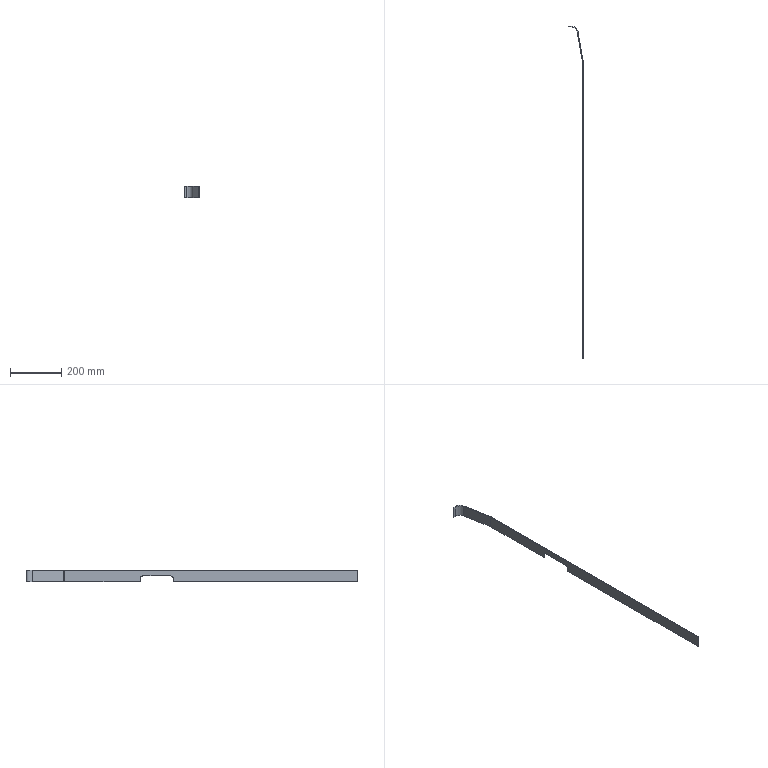Part | SolidWorks | features FlatPattern 1, ICE 1, SMBaseFlange 1, SheetMetal 1 | 1 solid | 28 faces | box 60.1 x 1293 x 45 mm | volume 180831 mm3 | plane 22 | cylinder 6 | commonest cylinder face diameters 20 x2 50 x2 56.4 x2
STEP:
#1=CARTESIAN_POINT('',(63.4,-447.3,-22.5));
#2=VERTEX_POINT('',#1);
#3=CARTESIAN_POINT('',(60.2,-447.3,-22.5));
#4=VERTEX_POINT('',#3);
#5=CARTESIAN_POINT('',(63.4,-447.3,-22.5));
#6=DIRECTION('',(-1.,0.,0.));
#7=VECTOR('',#6,1000.);
#8=LINE('',#5,#7);
#9=EDGE_CURVE('',#2,#4,#8,.T.);
#10=ORIENTED_EDGE('',*,*,#9,.T.);
#11=CARTESIAN_POINT('',(60.2,-153.273,-22.5));
#12=VERTEX_POINT('',#11);
#13=CARTESIAN_POINT('',(60.2,-153.273,-22.5));
#14=DIRECTION('',(0.,1.,0.));
#15=VECTOR('',#14,1000.);
#16=LINE('',#13,#15);
#17=EDGE_CURVE('',#4,#12,#16,.T.);
#18=ORIENTED_EDGE('',*,*,#17,.T.);
#19=CARTESIAN_POINT('',(63.4,-153.273,-22.5));
#20=VERTEX_POINT('',#19);
#21=CARTESIAN_POINT('',(60.2,-153.273,-22.5));
#22=DIRECTION('',(1.,0.,0.));
#23=VECTOR('',#22,1000.);
#24=LINE('',#21,#23);
#25=EDGE_CURVE('',#12,#20,#24,.T.);
#26=ORIENTED_EDGE('',*,*,#25,.T.);
#27=CARTESIAN_POINT('',(63.4,-153.273,-22.5));
#28=DIRECTION('',(0.,1.,0.));
#29=VECTOR('',#28,1000.);
#30=LINE('',#27,#29);
#31=EDGE_CURVE('',#2,#20,#30,.T.);
#32=ORIENTED_EDGE('',*,*,#31,.F.);
#33=EDGE_LOOP('',(#10,#18,#26,#32));
#34=FACE_OUTER_BOUND('',#33,.T.);
#35=CARTESIAN_POINT('',(62.97,-148.368,-22.5));
#36=DIRECTION('',(0.,0.,-1.));
#37=DIRECTION('',(-1.,0.,0.));
#38=AXIS2_PLACEMENT_3D('',#35,#36,#37);
#39=PLANE('',#38);
#40=ADVANCED_FACE('',(#34),#39,.T.);
#41=CARTESIAN_POINT('',(59.819,-148.925,22.5));
#42=VERTEX_POINT('',#41);
#43=CARTESIAN_POINT('',(62.97,-148.368,22.5));
#44=VERTEX_POINT('',#43);
#45=CARTESIAN_POINT('',(59.819,-148.925,22.5));
#46=DIRECTION('',(0.9848,0.1739,0.));
#47=VECTOR('',#46,1000.);
#48=LINE('',#45,#47);
#49=EDGE_CURVE('',#42,#44,#48,.T.);
#50=ORIENTED_EDGE('',*,*,#49,.F.);
#51=CARTESIAN_POINT('',(60.2,-153.273,22.5));
#52=VERTEX_POINT('',#51);
#53=CARTESIAN_POINT('',(35.2,-153.273,22.5));
#54=DIRECTION('',(0.,0.,1.));
#55=DIRECTION('',(-1.,0.,0.));
#56=AXIS2_PLACEMENT_3D('',#53,#54,#55);
#57=CIRCLE('',#56,25.);
#58=EDGE_CURVE('',#52,#42,#57,.T.);
#59=ORIENTED_EDGE('',*,*,#58,.F.);
#60=CARTESIAN_POINT('',(63.4,-153.273,22.5));
#61=VERTEX_POINT('',#60);
#62=CARTESIAN_POINT('',(63.4,-153.273,22.5));
#63=DIRECTION('',(-1.,0.,0.));
#64=VECTOR('',#63,1000.);
#65=LINE('',#62,#64);
#66=EDGE_CURVE('',#61,#52,#65,.T.);
#67=ORIENTED_EDGE('',*,*,#66,.F.);
#68=CARTESIAN_POINT('',(35.2,-153.273,22.5));
#69=DIRECTION('',(0.,0.,1.));
#70=DIRECTION('',(1.,0.,0.));
#71=AXIS2_PLACEMENT_3D('',#68,#69,#70);
#72=CIRCLE('',#71,28.2);
#73=EDGE_CURVE('',#61,#44,#72,.T.);
#74=ORIENTED_EDGE('',*,*,#73,.T.);
#75=EDGE_LOOP('',(#50,#59,#67,#74));
#76=FACE_OUTER_BOUND('',#75,.T.);
#77=CARTESIAN_POINT('',(59.819,-148.925,22.5));
#78=DIRECTION('',(0.,0.,1.));
#79=DIRECTION('',(1.,0.,0.));
#80=AXIS2_PLACEMENT_3D('',#77,#78,#79);
#81=PLANE('',#80);
#82=ADVANCED_FACE('',(#76),#81,.T.);
#83=CARTESIAN_POINT('',(38.134,-26.152,22.5));
#84=VERTEX_POINT('',#83);
#85=CARTESIAN_POINT('',(38.134,-26.152,22.5));
#86=DIRECTION('',(-0.1739,0.9848,0.));
#87=VECTOR('',#86,1000.);
#88=LINE('',#85,#87);
#89=EDGE_CURVE('',#42,#84,#88,.T.);
#90=ORIENTED_EDGE('',*,*,#89,.F.);
#91=ORIENTED_EDGE('',*,*,#49,.T.);
#92=CARTESIAN_POINT('',(41.285,-25.595,22.5));
#93=VERTEX_POINT('',#92);
#94=CARTESIAN_POINT('',(41.285,-25.595,22.5));
#95=DIRECTION('',(-0.1739,0.9848,0.));
#96=VECTOR('',#95,1000.);
#97=LINE('',#94,#96);
#98=EDGE_CURVE('',#44,#93,#97,.T.);
#99=ORIENTED_EDGE('',*,*,#98,.T.);
#100=CARTESIAN_POINT('',(41.285,-25.595,22.5));
#101=DIRECTION('',(-0.9848,-0.1739,0.));
#102=VECTOR('',#101,1000.);
#103=LINE('',#100,#102);
#104=EDGE_CURVE('',#93,#84,#103,.T.);
#105=ORIENTED_EDGE('',*,*,#104,.T.);
#106=EDGE_LOOP('',(#90,#91,#99,#105));
#107=FACE_OUTER_BOUND('',#106,.T.);
#108=CARTESIAN_POINT('',(63.4,-153.273,22.5));
#109=DIRECTION('',(0.,0.,1.));
#110=DIRECTION('',(1.,0.,0.));
#111=AXIS2_PLACEMENT_3D('',#108,#109,#110);
#112=PLANE('',#111);
#113=ADVANCED_FACE('',(#107),#112,.T.);
#114=ORIENTED_EDGE('',*,*,#25,.F.);
#115=CARTESIAN_POINT('',(59.819,-148.925,-22.5));
#116=VERTEX_POINT('',#115);
#117=CARTESIAN_POINT('',(35.2,-153.273,-22.5));
#118=DIRECTION('',(0.,0.,1.));
#119=DIRECTION('',(-1.,0.,0.));
#120=AXIS2_PLACEMENT_3D('',#117,#118,#119);
#121=CIRCLE('',#120,25.);
#122=EDGE_CURVE('',#12,#116,#121,.T.);
#123=ORIENTED_EDGE('',*,*,#122,.T.);
#124=CARTESIAN_POINT('',(62.97,-148.368,-22.5));
#125=VERTEX_POINT('',#124);
#126=CARTESIAN_POINT('',(62.97,-148.368,-22.5));
#127=DIRECTION('',(-0.9848,-0.1739,0.));
#128=VECTOR('',#127,1000.);
#129=LINE('',#126,#128);
#130=EDGE_CURVE('',#125,#116,#129,.T.);
#131=ORIENTED_EDGE('',*,*,#130,.F.);
#132=CARTESIAN_POINT('',(35.2,-153.273,-22.5));
#133=DIRECTION('',(0.,0.,1.));
#134=DIRECTION('',(1.,0.,0.));
#135=AXIS2_PLACEMENT_3D('',#132,#133,#134);
#136=CIRCLE('',#135,28.2);
#137=EDGE_CURVE('',#20,#125,#136,.T.);
#138=ORIENTED_EDGE('',*,*,#137,.F.);
#139=EDGE_LOOP('',(#114,#123,#131,#138));
#140=FACE_OUTER_BOUND('',#139,.T.);
#141=CARTESIAN_POINT('',(60.2,-153.273,-22.5));
#142=DIRECTION('',(0.,0.,-1.));
#143=DIRECTION('',(-1.,0.,0.));
#144=AXIS2_PLACEMENT_3D('',#141,#142,#143);
#145=PLANE('',#144);
#146=ADVANCED_FACE('',(#140),#145,.T.);
#147=CARTESIAN_POINT('',(63.4,-575.3,-22.5));
#148=VERTEX_POINT('',#147);
#149=CARTESIAN_POINT('',(60.2,-575.3,-22.5));
#150=VERTEX_POINT('',#149);
#151=CARTESIAN_POINT('',(63.4,-575.3,-22.5));
#152=DIRECTION('',(-1.,0.,0.));
#153=VECTOR('',#152,1000.);
#154=LINE('',#151,#153);
#155=EDGE_CURVE('',#148,#150,#154,.T.);
#156=ORIENTED_EDGE('',*,*,#155,.F.);
#157=CARTESIAN_POINT('',(63.4,-1295.7,-22.5));
#158=VERTEX_POINT('',#157);
#159=CARTESIAN_POINT('',(63.4,-153.273,-22.5));
#160=DIRECTION('',(0.,1.,0.));
#161=VECTOR('',#160,1000.);
#162=LINE('',#159,#161);
#163=EDGE_CURVE('',#158,#148,#162,.T.);
#164=ORIENTED_EDGE('',*,*,#163,.F.);
#165=CARTESIAN_POINT('',(60.2,-1295.7,-22.5));
#166=VERTEX_POINT('',#165);
#167=CARTESIAN_POINT('',(63.4,-1295.7,-22.5));
#168=DIRECTION('',(-1.,0.,0.));
#169=VECTOR('',#168,1000.);
#170=LINE('',#167,#169);
#171=EDGE_CURVE('',#158,#166,#170,.T.);
#172=ORIENTED_EDGE('',*,*,#171,.T.);
#173=CARTESIAN_POINT('',(60.2,-153.273,-22.5));
#174=DIRECTION('',(0.,1.,0.));
#175=VECTOR('',#174,1000.);
#176=LINE('',#173,#175);
#177=EDGE_CURVE('',#166,#150,#176,.T.);
#178=ORIENTED_EDGE('',*,*,#177,.T.);
#179=EDGE_LOOP('',(#156,#164,#172,#178));
#180=FACE_OUTER_BOUND('',#179,.T.);
#181=CARTESIAN_POINT('',(62.97,-148.368,-22.5));
#182=DIRECTION('',(0.,0.,-1.));
#183=DIRECTION('',(-1.,0.,0.));
#184=AXIS2_PLACEMENT_3D('',#181,#182,#183);
#185=PLANE('',#184);
#186=ADVANCED_FACE('',(#180),#185,.T.);
#187=CARTESIAN_POINT('',(13.515,-5.5,22.5));
#188=VERTEX_POINT('',#187);
#189=CARTESIAN_POINT('',(13.515,-2.3,22.5));
#190=VERTEX_POINT('',#189);
#191=CARTESIAN_POINT('',(13.515,-5.5,22.5));
#192=DIRECTION('',(0.,1.,0.));
#193=VECTOR('',#192,1000.);
#194=LINE('',#191,#193);
#195=EDGE_CURVE('',#188,#190,#194,.T.);
#196=ORIENTED_EDGE('',*,*,#195,.F.);
#197=CARTESIAN_POINT('',(13.515,-30.5,22.5));
#198=DIRECTION('',(0.,0.,1.));
#199=DIRECTION('',(-1.,0.,0.));
#200=AXIS2_PLACEMENT_3D('',#197,#198,#199);
#201=CIRCLE('',#200,25.);
#202=EDGE_CURVE('',#84,#188,#201,.T.);
#203=ORIENTED_EDGE('',*,*,#202,.F.);
#204=ORIENTED_EDGE('',*,*,#104,.F.);
#205=CARTESIAN_POINT('',(13.515,-30.5,22.5));
#206=DIRECTION('',(0.,0.,1.));
#207=DIRECTION('',(1.,0.,0.));
#208=AXIS2_PLACEMENT_3D('',#205,#206,#207);
#209=CIRCLE('',#208,28.2);
#210=EDGE_CURVE('',#93,#190,#209,.T.);
#211=ORIENTED_EDGE('',*,*,#210,.T.);
#212=EDGE_LOOP('',(#196,#203,#204,#211));
#213=FACE_OUTER_BOUND('',#212,.T.);
#214=CARTESIAN_POINT('',(13.515,-5.5,22.5));
#215=DIRECTION('',(0.,0.,1.));
#216=DIRECTION('',(1.,0.,0.));
#217=AXIS2_PLACEMENT_3D('',#214,#215,#216);
#218=PLANE('',#217);
#219=ADVANCED_FACE('',(#213),#218,.T.);
#220=CARTESIAN_POINT('',(3.3,-5.5,22.5));
#221=VERTEX_POINT('',#220);
#222=CARTESIAN_POINT('',(13.515,-5.5,22.5));
#223=DIRECTION('',(-1.,0.,0.));
#224=VECTOR('',#223,1000.);
#225=LINE('',#222,#224);
#226=EDGE_CURVE('',#188,#221,#225,.T.);
#227=ORIENTED_EDGE('',*,*,#226,.F.);
#228=ORIENTED_EDGE('',*,*,#195,.T.);
#229=CARTESIAN_POINT('',(3.3,-2.3,22.5));
#230=VERTEX_POINT('',#229);
#231=CARTESIAN_POINT('',(13.515,-2.3,22.5));
#232=DIRECTION('',(-1.,0.,0.));
#233=VECTOR('',#232,1000.);
#234=LINE('',#231,#233);
#235=EDGE_CURVE('',#190,#230,#234,.T.);
#236=ORIENTED_EDGE('',*,*,#235,.T.);
#237=CARTESIAN_POINT('',(3.3,-5.5,22.5));
#238=DIRECTION('',(0.,1.,0.));
#239=VECTOR('',#238,1000.);
#240=LINE('',#237,#239);
#241=EDGE_CURVE('',#221,#230,#240,.T.);
#242=ORIENTED_EDGE('',*,*,#241,.F.);
#243=EDGE_LOOP('',(#227,#228,#236,#242));
#244=FACE_OUTER_BOUND('',#243,.T.);
#245=CARTESIAN_POINT('',(41.285,-25.595,22.5));
#246=DIRECTION('',(0.,0.,1.));
#247=DIRECTION('',(1.,0.,0.));
#248=AXIS2_PLACEMENT_3D('',#245,#246,#247);
#249=PLANE('',#248);
#250=ADVANCED_FACE('',(#244),#249,.T.);
#251=CARTESIAN_POINT('',(38.134,-26.152,-22.5));
#252=VERTEX_POINT('',#251);
#253=CARTESIAN_POINT('',(41.285,-25.595,-22.5));
#254=VERTEX_POINT('',#253);
#255=CARTESIAN_POINT('',(38.134,-26.152,-22.5));
#256=DIRECTION('',(0.9848,0.1739,0.));
#257=VECTOR('',#256,1000.);
#258=LINE('',#255,#257);
#259=EDGE_CURVE('',#252,#254,#258,.T.);
#260=ORIENTED_EDGE('',*,*,#259,.F.);
#261=CARTESIAN_POINT('',(13.515,-5.5,-22.5));
#262=VERTEX_POINT('',#261);
#263=CARTESIAN_POINT('',(13.515,-30.5,-22.5));
#264=DIRECTION('',(0.,0.,1.));
#265=DIRECTION('',(-1.,0.,0.));
#266=AXIS2_PLACEMENT_3D('',#263,#264,#265);
#267=CIRCLE('',#266,25.);
#268=EDGE_CURVE('',#252,#262,#267,.T.);
#269=ORIENTED_EDGE('',*,*,#268,.T.);
#270=CARTESIAN_POINT('',(13.515,-2.3,-22.5));
#271=VERTEX_POINT('',#270);
#272=CARTESIAN_POINT('',(13.515,-2.3,-22.5));
#273=DIRECTION('',(0.,-1.,0.));
#274=VECTOR('',#273,1000.);
#275=LINE('',#272,#274);
#276=EDGE_CURVE('',#271,#262,#275,.T.);
#277=ORIENTED_EDGE('',*,*,#276,.F.);
#278=CARTESIAN_POINT('',(13.515,-30.5,-22.5));
#279=DIRECTION('',(0.,0.,1.));
#280=DIRECTION('',(1.,0.,0.));
#281=AXIS2_PLACEMENT_3D('',#278,#279,#280);
#282=CIRCLE('',#281,28.2);
#283=EDGE_CURVE('',#254,#271,#282,.T.);
#284=ORIENTED_EDGE('',*,*,#283,.F.);
#285=EDGE_LOOP('',(#260,#269,#277,#284));
#286=FACE_OUTER_BOUND('',#285,.T.);
#287=CARTESIAN_POINT('',(38.134,-26.152,-22.5));
#288=DIRECTION('',(0.,0.,-1.));
#289=DIRECTION('',(-1.,0.,0.));
#290=AXIS2_PLACEMENT_3D('',#287,#288,#289);
#291=PLANE('',#290);
#292=ADVANCED_FACE('',(#286),#291,.T.);
#293=CARTESIAN_POINT('',(38.134,-26.152,-22.5));
#294=DIRECTION('',(-0.1739,0.9848,0.));
#295=VECTOR('',#294,1000.);
#296=LINE('',#293,#295);
#297=EDGE_CURVE('',#116,#252,#296,.T.);
#298=ORIENTED_EDGE('',*,*,#297,.T.);
#299=ORIENTED_EDGE('',*,*,#259,.T.);
#300=CARTESIAN_POINT('',(41.285,-25.595,-22.5));
#301=DIRECTION('',(-0.1739,0.9848,0.));
#302=VECTOR('',#301,1000.);
#303=LINE('',#300,#302);
#304=EDGE_CURVE('',#125,#254,#303,.T.);
#305=ORIENTED_EDGE('',*,*,#304,.F.);
#306=ORIENTED_EDGE('',*,*,#130,.T.);
#307=EDGE_LOOP('',(#298,#299,#305,#306));
#308=FACE_OUTER_BOUND('',#307,.T.);
#309=CARTESIAN_POINT('',(13.515,-2.3,-22.5));
#310=DIRECTION('',(0.,0.,-1.));
#311=DIRECTION('',(-1.,0.,0.));
#312=AXIS2_PLACEMENT_3D('',#309,#310,#311);
#313=PLANE('',#312);
#314=ADVANCED_FACE('',(#308),#313,.T.);
#315=CARTESIAN_POINT('',(3.3,-2.3,-22.5));
#316=VERTEX_POINT('',#315);
#317=CARTESIAN_POINT('',(13.515,-2.3,-22.5));
#318=DIRECTION('',(-1.,0.,0.));
#319=VECTOR('',#318,1000.);
#320=LINE('',#317,#319);
#321=EDGE_CURVE('',#271,#316,#320,.T.);
#322=ORIENTED_EDGE('',*,*,#321,.T.);
#323=CARTESIAN_POINT('',(3.3,-2.3,22.5));
#324=DIRECTION('',(0.,0.,-1.));
#325=VECTOR('',#324,1000.);
#326=LINE('',#323,#325);
#327=EDGE_CURVE('',#230,#316,#326,.T.);
#328=ORIENTED_EDGE('',*,*,#327,.F.);
#329=ORIENTED_EDGE('',*,*,#235,.F.);
#330=CARTESIAN_POINT('',(13.515,-2.3,22.5));
#331=DIRECTION('',(0.,0.,-1.));
#332=VECTOR('',#331,1000.);
#333=LINE('',#330,#332);
#334=EDGE_CURVE('',#190,#271,#333,.T.);
#335=ORIENTED_EDGE('',*,*,#334,.T.);
#336=EDGE_LOOP('',(#322,#328,#329,#335));
#337=FACE_OUTER_BOUND('',#336,.T.);
#338=CARTESIAN_POINT('',(13.515,-2.3,22.5));
#339=DIRECTION('',(0.,-1.,0.));
#340=DIRECTION('',(1.,0.,0.));
#341=AXIS2_PLACEMENT_3D('',#338,#339,#340);
#342=PLANE('',#341);
#343=ADVANCED_FACE('',(#337),#342,.F.);
#344=CARTESIAN_POINT('',(3.3,-5.5,-22.5));
#345=VERTEX_POINT('',#344);
#346=CARTESIAN_POINT('',(3.3,-5.5,-22.5));
#347=DIRECTION('',(0.,1.,0.));
#348=VECTOR('',#347,1000.);
#349=LINE('',#346,#348);
#350=EDGE_CURVE('',#345,#316,#349,.T.);
#351=ORIENTED_EDGE('',*,*,#350,.F.);
#352=CARTESIAN_POINT('',(3.3,-5.5,22.5));
#353=DIRECTION('',(0.,0.,-1.));
#354=VECTOR('',#353,1000.);
#355=LINE('',#352,#354);
#356=EDGE_CURVE('',#221,#345,#355,.T.);
#357=ORIENTED_EDGE('',*,*,#356,.F.);
#358=ORIENTED_EDGE('',*,*,#241,.T.);
#359=ORIENTED_EDGE('',*,*,#327,.T.);
#360=EDGE_LOOP('',(#351,#357,#358,#359));
#361=FACE_OUTER_BOUND('',#360,.T.);
#362=CARTESIAN_POINT('',(3.3,-5.5,22.5));
#363=DIRECTION('',(-1.,0.,0.));
#364=DIRECTION('',(0.,0.,1.));
#365=AXIS2_PLACEMENT_3D('',#362,#363,#364);
#366=PLANE('',#365);
#367=ADVANCED_FACE('',(#361),#366,.T.);
#368=CARTESIAN_POINT('',(13.515,-5.5,-22.5));
#369=DIRECTION('',(-1.,0.,0.));
#370=VECTOR('',#369,1000.);
#371=LINE('',#368,#370);
#372=EDGE_CURVE('',#262,#345,#371,.T.);
#373=ORIENTED_EDGE('',*,*,#372,.F.);
#374=CARTESIAN_POINT('',(13.515,-5.5,22.5));
#375=DIRECTION('',(0.,0.,-1.));
#376=VECTOR('',#375,1000.);
#377=LINE('',#374,#376);
#378=EDGE_CURVE('',#188,#262,#377,.T.);
#379=ORIENTED_EDGE('',*,*,#378,.F.);
#380=ORIENTED_EDGE('',*,*,#226,.T.);
#381=ORIENTED_EDGE('',*,*,#356,.T.);
#382=EDGE_LOOP('',(#373,#379,#380,#381));
#383=FACE_OUTER_BOUND('',#382,.T.);
#384=CARTESIAN_POINT('',(13.515,-5.5,22.5));
#385=DIRECTION('',(0.,-1.,0.));
#386=DIRECTION('',(1.,0.,0.));
#387=AXIS2_PLACEMENT_3D('',#384,#385,#386);
#388=PLANE('',#387);
#389=ADVANCED_FACE('',(#383),#388,.T.);
#390=ORIENTED_EDGE('',*,*,#268,.F.);
#391=CARTESIAN_POINT('',(38.134,-26.152,22.5));
#392=DIRECTION('',(0.,0.,-1.));
#393=VECTOR('',#392,1000.);
#394=LINE('',#391,#393);
#395=EDGE_CURVE('',#84,#252,#394,.T.);
#396=ORIENTED_EDGE('',*,*,#395,.F.);
#397=ORIENTED_EDGE('',*,*,#202,.T.);
#398=ORIENTED_EDGE('',*,*,#378,.T.);
#399=EDGE_LOOP('',(#390,#396,#397,#398));
#400=FACE_OUTER_BOUND('',#399,.T.);
#401=CARTESIAN_POINT('',(13.515,-30.5,22.5));
#402=DIRECTION('',(0.,0.,-1.));
#403=DIRECTION('',(-1.,0.,0.));
#404=AXIS2_PLACEMENT_3D('',#401,#402,#403);
#405=CYLINDRICAL_SURFACE('',#404,25.);
#406=ADVANCED_FACE('',(#400),#405,.F.);
#407=ORIENTED_EDGE('',*,*,#297,.F.);
#408=CARTESIAN_POINT('',(59.819,-148.925,22.5));
#409=DIRECTION('',(0.,0.,-1.));
#410=VECTOR('',#409,1000.);
#411=LINE('',#408,#410);
#412=EDGE_CURVE('',#42,#116,#411,.T.);
#413=ORIENTED_EDGE('',*,*,#412,.F.);
#414=ORIENTED_EDGE('',*,*,#89,.T.);
#415=ORIENTED_EDGE('',*,*,#395,.T.);
#416=EDGE_LOOP('',(#407,#413,#414,#415));
#417=FACE_OUTER_BOUND('',#416,.T.);
#418=CARTESIAN_POINT('',(38.134,-26.152,22.5));
#419=DIRECTION('',(-0.9848,-0.1739,0.));
#420=DIRECTION('',(0.1739,-0.9848,0.));
#421=AXIS2_PLACEMENT_3D('',#418,#419,#420);
#422=PLANE('',#421);
#423=ADVANCED_FACE('',(#417),#422,.T.);
#424=ORIENTED_EDGE('',*,*,#122,.F.);
#425=CARTESIAN_POINT('',(60.2,-153.273,22.5));
#426=DIRECTION('',(0.,0.,-1.));
#427=VECTOR('',#426,1000.);
#428=LINE('',#425,#427);
#429=EDGE_CURVE('',#52,#12,#428,.T.);
#430=ORIENTED_EDGE('',*,*,#429,.F.);
#431=ORIENTED_EDGE('',*,*,#58,.T.);
#432=ORIENTED_EDGE('',*,*,#412,.T.);
#433=EDGE_LOOP('',(#424,#430,#431,#432));
#434=FACE_OUTER_BOUND('',#433,.T.);
#435=CARTESIAN_POINT('',(35.2,-153.273,22.5));
#436=DIRECTION('',(0.,0.,-1.));
#437=DIRECTION('',(-1.,0.,0.));
#438=AXIS2_PLACEMENT_3D('',#435,#436,#437);
#439=CYLINDRICAL_SURFACE('',#438,25.);
#440=ADVANCED_FACE('',(#434),#439,.F.);
#441=CARTESIAN_POINT('',(60.2,-447.3,-9.9));
#442=VERTEX_POINT('',#441);
#443=CARTESIAN_POINT('',(60.2,-447.3,-9.9));
#444=DIRECTION('',(0.,0.,-1.));
#445=VECTOR('',#444,1000.);
#446=LINE('',#443,#445);
#447=EDGE_CURVE('',#442,#4,#446,.T.);
#448=ORIENTED_EDGE('',*,*,#447,.F.);
#449=CARTESIAN_POINT('',(60.2,-457.3,0.1));
#450=VERTEX_POINT('',#449);
#451=CARTESIAN_POINT('',(60.2,-457.3,-9.9));
#452=DIRECTION('',(-1.,0.,0.));
#453=DIRECTION('',(0.,-1.,0.));
#454=AXIS2_PLACEMENT_3D('',#451,#452,#453);
#455=CIRCLE('',#454,10.);
#456=EDGE_CURVE('',#450,#442,#455,.T.);
#457=ORIENTED_EDGE('',*,*,#456,.F.);
#458=CARTESIAN_POINT('',(60.2,-565.3,0.1));
#459=VERTEX_POINT('',#458);
#460=CARTESIAN_POINT('',(60.2,-457.3,0.1));
#461=DIRECTION('',(0.,1.,0.));
#462=VECTOR('',#461,1000.);
#463=LINE('',#460,#462);
#464=EDGE_CURVE('',#459,#450,#463,.T.);
#465=ORIENTED_EDGE('',*,*,#464,.F.);
#466=CARTESIAN_POINT('',(60.2,-575.3,-9.9));
#467=VERTEX_POINT('',#466);
#468=CARTESIAN_POINT('',(60.2,-565.3,-9.9));
#469=DIRECTION('',(-1.,0.,0.));
#470=DIRECTION('',(0.,1.,0.));
#471=AXIS2_PLACEMENT_3D('',#468,#469,#470);
#472=CIRCLE('',#471,10.);
#473=EDGE_CURVE('',#467,#459,#472,.T.);
#474=ORIENTED_EDGE('',*,*,#473,.F.);
#475=CARTESIAN_POINT('',(60.2,-575.3,-22.5));
#476=DIRECTION('',(0.,0.,1.));
#477=VECTOR('',#476,1000.);
#478=LINE('',#475,#477);
#479=EDGE_CURVE('',#150,#467,#478,.T.);
#480=ORIENTED_EDGE('',*,*,#479,.F.);
#481=ORIENTED_EDGE('',*,*,#177,.F.);
#482=CARTESIAN_POINT('',(60.2,-1295.7,22.5));
#483=VERTEX_POINT('',#482);
#484=CARTESIAN_POINT('',(60.2,-1295.7,22.5));
#485=DIRECTION('',(0.,0.,-1.));
#486=VECTOR('',#485,1000.);
#487=LINE('',#484,#486);
#488=EDGE_CURVE('',#483,#166,#487,.T.);
#489=ORIENTED_EDGE('',*,*,#488,.F.);
#490=CARTESIAN_POINT('',(60.2,-153.273,22.5));
#491=DIRECTION('',(0.,1.,0.));
#492=VECTOR('',#491,1000.);
#493=LINE('',#490,#492);
#494=EDGE_CURVE('',#483,#52,#493,.T.);
#495=ORIENTED_EDGE('',*,*,#494,.T.);
#496=ORIENTED_EDGE('',*,*,#429,.T.);
#497=ORIENTED_EDGE('',*,*,#17,.F.);
#498=EDGE_LOOP('',(#448,#457,#465,#474,#480,#481,#489,#495,#496,#497));
#499=FACE_OUTER_BOUND('',#498,.T.);
#500=CARTESIAN_POINT('',(60.2,-153.273,22.5));
#501=DIRECTION('',(-1.,0.,0.));
#502=DIRECTION('',(0.,-1.,0.));
#503=AXIS2_PLACEMENT_3D('',#500,#501,#502);
#504=PLANE('',#503);
#505=ADVANCED_FACE('',(#499),#504,.T.);
#506=ORIENTED_EDGE('',*,*,#171,.F.);
#507=CARTESIAN_POINT('',(63.4,-1295.7,22.5));
#508=VERTEX_POINT('',#507);
#509=CARTESIAN_POINT('',(63.4,-1295.7,22.5));
#510=DIRECTION('',(0.,0.,-1.));
#511=VECTOR('',#510,1000.);
#512=LINE('',#509,#511);
#513=EDGE_CURVE('',#508,#158,#512,.T.);
#514=ORIENTED_EDGE('',*,*,#513,.F.);
#515=CARTESIAN_POINT('',(63.4,-1295.7,22.5));
#516=DIRECTION('',(-1.,0.,0.));
#517=VECTOR('',#516,1000.);
#518=LINE('',#515,#517);
#519=EDGE_CURVE('',#508,#483,#518,.T.);
#520=ORIENTED_EDGE('',*,*,#519,.T.);
#521=ORIENTED_EDGE('',*,*,#488,.T.);
#522=EDGE_LOOP('',(#506,#514,#520,#521));
#523=FACE_OUTER_BOUND('',#522,.T.);
#524=CARTESIAN_POINT('',(63.4,-1295.7,22.5));
#525=DIRECTION('',(0.,-1.,0.));
#526=DIRECTION('',(0.,0.,-1.));
#527=AXIS2_PLACEMENT_3D('',#524,#525,#526);
#528=PLANE('',#527);
#529=ADVANCED_FACE('',(#523),#528,.T.);
#530=CARTESIAN_POINT('',(63.4,-457.3,0.1));
#531=VERTEX_POINT('',#530);
#532=CARTESIAN_POINT('',(63.4,-447.3,-9.9));
#533=VERTEX_POINT('',#532);
#534=CARTESIAN_POINT('',(63.4,-457.3,-9.9));
#535=DIRECTION('',(-1.,0.,0.));
#536=DIRECTION('',(0.,-1.,0.));
#537=AXIS2_PLACEMENT_3D('',#534,#535,#536);
#538=CIRCLE('',#537,10.);
#539=EDGE_CURVE('',#531,#533,#538,.T.);
#540=ORIENTED_EDGE('',*,*,#539,.T.);
#541=CARTESIAN_POINT('',(63.4,-447.3,-9.9));
#542=DIRECTION('',(0.,0.,-1.));
#543=VECTOR('',#542,1000.);
#544=LINE('',#541,#543);
#545=EDGE_CURVE('',#533,#2,#544,.T.);
#546=ORIENTED_EDGE('',*,*,#545,.T.);
#547=ORIENTED_EDGE('',*,*,#31,.T.);
#548=CARTESIAN_POINT('',(63.4,-153.273,22.5));
#549=DIRECTION('',(0.,0.,-1.));
#550=VECTOR('',#549,1000.);
#551=LINE('',#548,#550);
#552=EDGE_CURVE('',#61,#20,#551,.T.);
#553=ORIENTED_EDGE('',*,*,#552,.F.);
#554=CARTESIAN_POINT('',(63.4,-153.273,22.5));
#555=DIRECTION('',(0.,1.,0.));
#556=VECTOR('',#555,1000.);
#557=LINE('',#554,#556);
#558=EDGE_CURVE('',#508,#61,#557,.T.);
#559=ORIENTED_EDGE('',*,*,#558,.F.);
#560=ORIENTED_EDGE('',*,*,#513,.T.);
#561=ORIENTED_EDGE('',*,*,#163,.T.);
#562=CARTESIAN_POINT('',(63.4,-575.3,-9.9));
#563=VERTEX_POINT('',#562);
#564=CARTESIAN_POINT('',(63.4,-575.3,-22.5));
#565=DIRECTION('',(0.,0.,1.));
#566=VECTOR('',#565,1000.);
#567=LINE('',#564,#566);
#568=EDGE_CURVE('',#148,#563,#567,.T.);
#569=ORIENTED_EDGE('',*,*,#568,.T.);
#570=CARTESIAN_POINT('',(63.4,-565.3,0.1));
#571=VERTEX_POINT('',#570);
#572=CARTESIAN_POINT('',(63.4,-565.3,-9.9));
#573=DIRECTION('',(-1.,0.,0.));
#574=DIRECTION('',(0.,1.,0.));
#575=AXIS2_PLACEMENT_3D('',#572,#573,#574);
#576=CIRCLE('',#575,10.);
#577=EDGE_CURVE('',#563,#571,#576,.T.);
#578=ORIENTED_EDGE('',*,*,#577,.T.);
#579=CARTESIAN_POINT('',(63.4,-457.3,0.1));
#580=DIRECTION('',(0.,1.,0.));
#581=VECTOR('',#580,1000.);
#582=LINE('',#579,#581);
#583=EDGE_CURVE('',#571,#531,#582,.T.);
#584=ORIENTED_EDGE('',*,*,#583,.T.);
#585=EDGE_LOOP('',(#540,#546,#547,#553,#559,#560,#561,#569,#578,#584));
#586=FACE_OUTER_BOUND('',#585,.T.);
#587=CARTESIAN_POINT('',(63.4,-153.273,22.5));
#588=DIRECTION('',(-1.,0.,0.));
#589=DIRECTION('',(0.,-1.,0.));
#590=AXIS2_PLACEMENT_3D('',#587,#588,#589);
#591=PLANE('',#590);
#592=ADVANCED_FACE('',(#586),#591,.F.);
#593=ORIENTED_EDGE('',*,*,#137,.T.);
#594=CARTESIAN_POINT('',(62.97,-148.368,22.5));
#595=DIRECTION('',(0.,0.,-1.));
#596=VECTOR('',#595,1000.);
#597=LINE('',#594,#596);
#598=EDGE_CURVE('',#44,#125,#597,.T.);
#599=ORIENTED_EDGE('',*,*,#598,.F.);
#600=ORIENTED_EDGE('',*,*,#73,.F.);
#601=ORIENTED_EDGE('',*,*,#552,.T.);
#602=EDGE_LOOP('',(#593,#599,#600,#601));
#603=FACE_OUTER_BOUND('',#602,.T.);
#604=CARTESIAN_POINT('',(35.2,-153.273,22.5));
#605=DIRECTION('',(0.,0.,-1.));
#606=DIRECTION('',(-1.,0.,0.));
#607=AXIS2_PLACEMENT_3D('',#604,#605,#606);
#608=CYLINDRICAL_SURFACE('',#607,28.2);
#609=ADVANCED_FACE('',(#603),#608,.T.);
#610=ORIENTED_EDGE('',*,*,#304,.T.);
#611=CARTESIAN_POINT('',(41.285,-25.595,22.5));
#612=DIRECTION('',(0.,0.,-1.));
#613=VECTOR('',#612,1000.);
#614=LINE('',#611,#613);
#615=EDGE_CURVE('',#93,#254,#614,.T.);
#616=ORIENTED_EDGE('',*,*,#615,.F.);
#617=ORIENTED_EDGE('',*,*,#98,.F.);
#618=ORIENTED_EDGE('',*,*,#598,.T.);
#619=EDGE_LOOP('',(#610,#616,#617,#618));
#620=FACE_OUTER_BOUND('',#619,.T.);
#621=CARTESIAN_POINT('',(41.285,-25.595,22.5));
#622=DIRECTION('',(-0.9848,-0.1739,0.));
#623=DIRECTION('',(0.1739,-0.9848,0.));
#624=AXIS2_PLACEMENT_3D('',#621,#622,#623);
#625=PLANE('',#624);
#626=ADVANCED_FACE('',(#620),#625,.F.);
#627=ORIENTED_EDGE('',*,*,#283,.T.);
#628=ORIENTED_EDGE('',*,*,#334,.F.);
#629=ORIENTED_EDGE('',*,*,#210,.F.);
#630=ORIENTED_EDGE('',*,*,#615,.T.);
#631=EDGE_LOOP('',(#627,#628,#629,#630));
#632=FACE_OUTER_BOUND('',#631,.T.);
#633=CARTESIAN_POINT('',(13.515,-30.5,22.5));
#634=DIRECTION('',(0.,0.,-1.));
#635=DIRECTION('',(-1.,0.,0.));
#636=AXIS2_PLACEMENT_3D('',#633,#634,#635);
#637=CYLINDRICAL_SURFACE('',#636,28.2);
#638=ADVANCED_FACE('',(#632),#637,.T.);
#639=ORIENTED_EDGE('',*,*,#558,.T.);
#640=ORIENTED_EDGE('',*,*,#66,.T.);
#641=ORIENTED_EDGE('',*,*,#494,.F.);
#642=ORIENTED_EDGE('',*,*,#519,.F.);
#643=EDGE_LOOP('',(#639,#640,#641,#642));
#644=FACE_OUTER_BOUND('',#643,.T.);
#645=CARTESIAN_POINT('',(13.515,-30.5,22.5));
#646=DIRECTION('',(0.,0.,1.));
#647=DIRECTION('',(1.,0.,0.));
#648=AXIS2_PLACEMENT_3D('',#645,#646,#647);
#649=PLANE('',#648);
#650=ADVANCED_FACE('',(#644),#649,.T.);
#651=ORIENTED_EDGE('',*,*,#321,.F.);
#652=ORIENTED_EDGE('',*,*,#276,.T.);
#653=ORIENTED_EDGE('',*,*,#372,.T.);
#654=ORIENTED_EDGE('',*,*,#350,.T.);
#655=EDGE_LOOP('',(#651,#652,#653,#654));
#656=FACE_OUTER_BOUND('',#655,.T.);
#657=CARTESIAN_POINT('',(13.515,-30.5,-22.5));
#658=DIRECTION('',(0.,0.,1.));
#659=DIRECTION('',(1.,0.,0.));
#660=AXIS2_PLACEMENT_3D('',#657,#658,#659);
#661=PLANE('',#660);
#662=ADVANCED_FACE('',(#656),#661,.F.);
#663=ORIENTED_EDGE('',*,*,#447,.T.);
#664=ORIENTED_EDGE('',*,*,#9,.F.);
#665=ORIENTED_EDGE('',*,*,#545,.F.);
#666=CARTESIAN_POINT('',(63.4,-447.3,-9.9));
#667=DIRECTION('',(-1.,0.,0.));
#668=VECTOR('',#667,1000.);
#669=LINE('',#666,#668);
#670=EDGE_CURVE('',#533,#442,#669,.T.);
#671=ORIENTED_EDGE('',*,*,#670,.T.);
#672=EDGE_LOOP('',(#663,#664,#665,#671));
#673=FACE_OUTER_BOUND('',#672,.T.);
#674=CARTESIAN_POINT('',(63.4,-447.3,-9.9));
#675=DIRECTION('',(0.,1.,0.));
#676=DIRECTION('',(-1.,0.,0.));
#677=AXIS2_PLACEMENT_3D('',#674,#675,#676);
#678=PLANE('',#677);
#679=ADVANCED_FACE('',(#673),#678,.F.);
#680=ORIENTED_EDGE('',*,*,#456,.T.);
#681=ORIENTED_EDGE('',*,*,#670,.F.);
#682=ORIENTED_EDGE('',*,*,#539,.F.);
#683=CARTESIAN_POINT('',(63.4,-457.3,0.1));
#684=DIRECTION('',(-1.,0.,0.));
#685=VECTOR('',#684,1000.);
#686=LINE('',#683,#685);
#687=EDGE_CURVE('',#531,#450,#686,.T.);
#688=ORIENTED_EDGE('',*,*,#687,.T.);
#689=EDGE_LOOP('',(#680,#681,#682,#688));
#690=FACE_OUTER_BOUND('',#689,.T.);
#691=CARTESIAN_POINT('',(63.4,-457.3,-9.9));
#692=DIRECTION('',(-1.,0.,0.));
#693=DIRECTION('',(0.,-1.,0.));
#694=AXIS2_PLACEMENT_3D('',#691,#692,#693);
#695=CYLINDRICAL_SURFACE('',#694,10.);
#696=ADVANCED_FACE('',(#690),#695,.F.);
#697=ORIENTED_EDGE('',*,*,#464,.T.);
#698=ORIENTED_EDGE('',*,*,#687,.F.);
#699=ORIENTED_EDGE('',*,*,#583,.F.);
#700=CARTESIAN_POINT('',(63.4,-565.3,0.1));
#701=DIRECTION('',(-1.,0.,0.));
#702=VECTOR('',#701,1000.);
#703=LINE('',#700,#702);
#704=EDGE_CURVE('',#571,#459,#703,.T.);
#705=ORIENTED_EDGE('',*,*,#704,.T.);
#706=EDGE_LOOP('',(#697,#698,#699,#705));
#707=FACE_OUTER_BOUND('',#706,.T.);
#708=CARTESIAN_POINT('',(63.4,-457.3,0.1));
#709=DIRECTION('',(0.,0.,1.));
#710=DIRECTION('',(0.,-1.,0.));
#711=AXIS2_PLACEMENT_3D('',#708,#709,#710);
#712=PLANE('',#711);
#713=ADVANCED_FACE('',(#707),#712,.F.);
#714=ORIENTED_EDGE('',*,*,#473,.T.);
#715=ORIENTED_EDGE('',*,*,#704,.F.);
#716=ORIENTED_EDGE('',*,*,#577,.F.);
#717=CARTESIAN_POINT('',(63.4,-575.3,-9.9));
#718=DIRECTION('',(-1.,0.,0.));
#719=VECTOR('',#718,1000.);
#720=LINE('',#717,#719);
#721=EDGE_CURVE('',#563,#467,#720,.T.);
#722=ORIENTED_EDGE('',*,*,#721,.T.);
#723=EDGE_LOOP('',(#714,#715,#716,#722));
#724=FACE_OUTER_BOUND('',#723,.T.);
#725=CARTESIAN_POINT('',(63.4,-565.3,-9.9));
#726=DIRECTION('',(-1.,0.,0.));
#727=DIRECTION('',(0.,-1.,0.));
#728=AXIS2_PLACEMENT_3D('',#725,#726,#727);
#729=CYLINDRICAL_SURFACE('',#728,10.);
#730=ADVANCED_FACE('',(#724),#729,.F.);
#731=ORIENTED_EDGE('',*,*,#479,.T.);
#732=ORIENTED_EDGE('',*,*,#721,.F.);
#733=ORIENTED_EDGE('',*,*,#568,.F.);
#734=ORIENTED_EDGE('',*,*,#155,.T.);
#735=EDGE_LOOP('',(#731,#732,#733,#734));
#736=FACE_OUTER_BOUND('',#735,.T.);
#737=CARTESIAN_POINT('',(63.4,-575.3,-22.5));
#738=DIRECTION('',(0.,-1.,0.));
#739=DIRECTION('',(0.,0.,-1.));
#740=AXIS2_PLACEMENT_3D('',#737,#738,#739);
#741=PLANE('',#740);
#742=ADVANCED_FACE('',(#736),#741,.F.);
#743=CLOSED_SHELL('',(#40,#82,#113,#146,#186,#219,#250,#292,#314,#343,#367,#389,#406,#423,#440,#505,#529,#592,#609,#626,#638,#650,#662,#679,#696,#713,#730,#742));
#744=MANIFOLD_SOLID_BREP('',#743);
#745=CARTESIAN_POINT('',(0.,0.,0.));
#746=DIRECTION('',(0.,0.,1.));
#747=DIRECTION('',(1.,0.,0.));
#748=AXIS2_PLACEMENT_3D('',#745,#746,#747);
#749=(LENGTH_UNIT()NAMED_UNIT(*)SI_UNIT(.MILLI.,.METRE.));
#750=UNCERTAINTY_MEASURE_WITH_UNIT(LENGTH_MEASURE(0.00001),#749,'','');
#751=(NAMED_UNIT(*)PLANE_ANGLE_UNIT()SI_UNIT($,.RADIAN.));
#752=(NAMED_UNIT(*)SI_UNIT($,.STERADIAN.)SOLID_ANGLE_UNIT());
#753=(GEOMETRIC_REPRESENTATION_CONTEXT(3)GLOBAL_UNCERTAINTY_ASSIGNED_CONTEXT((#750))GLOBAL_UNIT_ASSIGNED_CONTEXT((#749,#751,#752))REPRESENTATION_CONTEXT('',''));
#754=ADVANCED_BREP_SHAPE_REPRESENTATION('',(#744,#748),#753);